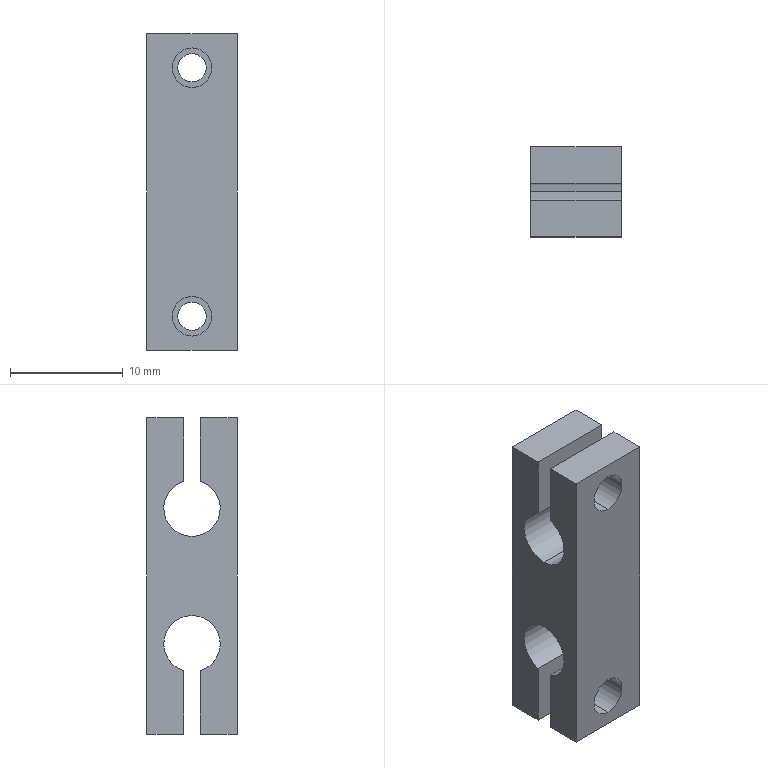Part | STEP file | 06-01-17 laser rotary plate B | 1 solid | 23 faces | box 8 x 8 x 28 mm | volume 1250 mm3 | plane 12 | cylinder 11 | commonest cylinder face diameters 2.5 x4 3.5 x4 5 x3
STEP:
#1=CARTESIAN_POINT('',(0.,0.75,1.75));
#2=VERTEX_POINT('',#1);
#3=CARTESIAN_POINT('',(0.,0.75,4.25));
#4=VERTEX_POINT('',#3);
#5=CARTESIAN_POINT('',(0.,0.75,3.));
#6=DIRECTION('',(0.,1.,0.));
#7=DIRECTION('',(0.,0.,1.));
#8=AXIS2_PLACEMENT_3D('',#5,#6,#7);
#9=CIRCLE('',#8,1.25);
#10=EDGE_CURVE('',#2,#4,#9,.T.);
#11=ORIENTED_EDGE('',*,*,#10,.F.);
#12=CARTESIAN_POINT('',(0.,4.,1.75));
#13=VERTEX_POINT('',#12);
#14=CARTESIAN_POINT('',(0.,4.,1.75));
#15=DIRECTION('',(0.,1.,0.));
#16=VECTOR('',#15,1000.);
#17=LINE('',#14,#16);
#18=EDGE_CURVE('',#2,#13,#17,.T.);
#19=ORIENTED_EDGE('',*,*,#18,.T.);
#20=CARTESIAN_POINT('',(0.,4.,4.25));
#21=VERTEX_POINT('',#20);
#22=CARTESIAN_POINT('',(0.,4.,3.));
#23=DIRECTION('',(0.,1.,0.));
#24=DIRECTION('',(0.,0.,1.));
#25=AXIS2_PLACEMENT_3D('',#22,#23,#24);
#26=CIRCLE('',#25,1.25);
#27=EDGE_CURVE('',#13,#21,#26,.T.);
#28=ORIENTED_EDGE('',*,*,#27,.T.);
#29=CARTESIAN_POINT('',(0.,4.,4.25));
#30=DIRECTION('',(0.,1.,0.));
#31=VECTOR('',#30,1000.);
#32=LINE('',#29,#31);
#33=EDGE_CURVE('',#4,#21,#32,.T.);
#34=ORIENTED_EDGE('',*,*,#33,.F.);
#35=EDGE_LOOP('',(#11,#19,#28,#34));
#36=FACE_OUTER_BOUND('',#35,.T.);
#37=CARTESIAN_POINT('',(0.,4.,3.));
#38=DIRECTION('',(0.,1.,0.));
#39=DIRECTION('',(0.,0.,1.));
#40=AXIS2_PLACEMENT_3D('',#37,#38,#39);
#41=CYLINDRICAL_SURFACE('',#40,1.25);
#42=ADVANCED_FACE('',(#36),#41,.F.);
#43=CARTESIAN_POINT('',(0.,0.75,23.75));
#44=VERTEX_POINT('',#43);
#45=CARTESIAN_POINT('',(0.,0.75,26.25));
#46=VERTEX_POINT('',#45);
#47=CARTESIAN_POINT('',(0.,0.75,25.));
#48=DIRECTION('',(0.,1.,0.));
#49=DIRECTION('',(0.,0.,1.));
#50=AXIS2_PLACEMENT_3D('',#47,#48,#49);
#51=CIRCLE('',#50,1.25);
#52=EDGE_CURVE('',#44,#46,#51,.T.);
#53=ORIENTED_EDGE('',*,*,#52,.F.);
#54=CARTESIAN_POINT('',(0.,4.,23.75));
#55=VERTEX_POINT('',#54);
#56=CARTESIAN_POINT('',(0.,4.,23.75));
#57=DIRECTION('',(0.,1.,0.));
#58=VECTOR('',#57,1000.);
#59=LINE('',#56,#58);
#60=EDGE_CURVE('',#44,#55,#59,.T.);
#61=ORIENTED_EDGE('',*,*,#60,.T.);
#62=CARTESIAN_POINT('',(0.,4.,26.25));
#63=VERTEX_POINT('',#62);
#64=CARTESIAN_POINT('',(0.,4.,25.));
#65=DIRECTION('',(0.,1.,0.));
#66=DIRECTION('',(0.,0.,1.));
#67=AXIS2_PLACEMENT_3D('',#64,#65,#66);
#68=CIRCLE('',#67,1.25);
#69=EDGE_CURVE('',#55,#63,#68,.T.);
#70=ORIENTED_EDGE('',*,*,#69,.T.);
#71=CARTESIAN_POINT('',(0.,4.,26.25));
#72=DIRECTION('',(0.,1.,0.));
#73=VECTOR('',#72,1000.);
#74=LINE('',#71,#73);
#75=EDGE_CURVE('',#46,#63,#74,.T.);
#76=ORIENTED_EDGE('',*,*,#75,.F.);
#77=EDGE_LOOP('',(#53,#61,#70,#76));
#78=FACE_OUTER_BOUND('',#77,.T.);
#79=CARTESIAN_POINT('',(0.,4.,25.));
#80=DIRECTION('',(0.,1.,0.));
#81=DIRECTION('',(0.,0.,1.));
#82=AXIS2_PLACEMENT_3D('',#79,#80,#81);
#83=CYLINDRICAL_SURFACE('',#82,1.25);
#84=ADVANCED_FACE('',(#78),#83,.F.);
#85=CARTESIAN_POINT('',(0.,-0.75,26.75));
#86=VERTEX_POINT('',#85);
#87=CARTESIAN_POINT('',(0.,-0.75,23.25));
#88=VERTEX_POINT('',#87);
#89=CARTESIAN_POINT('',(0.,-0.75,25.));
#90=DIRECTION('',(0.,-1.,0.));
#91=DIRECTION('',(0.,0.,-1.));
#92=AXIS2_PLACEMENT_3D('',#89,#90,#91);
#93=CIRCLE('',#92,1.75);
#94=EDGE_CURVE('',#86,#88,#93,.T.);
#95=ORIENTED_EDGE('',*,*,#94,.F.);
#96=CARTESIAN_POINT('',(0.,-4.,26.75));
#97=VERTEX_POINT('',#96);
#98=CARTESIAN_POINT('',(0.,0.,26.75));
#99=DIRECTION('',(0.,-1.,0.));
#100=VECTOR('',#99,1000.);
#101=LINE('',#98,#100);
#102=EDGE_CURVE('',#86,#97,#101,.T.);
#103=ORIENTED_EDGE('',*,*,#102,.T.);
#104=CARTESIAN_POINT('',(0.,-4.,23.25));
#105=VERTEX_POINT('',#104);
#106=CARTESIAN_POINT('',(0.,-4.,25.));
#107=DIRECTION('',(0.,-1.,0.));
#108=DIRECTION('',(0.,0.,1.));
#109=AXIS2_PLACEMENT_3D('',#106,#107,#108);
#110=CIRCLE('',#109,1.75);
#111=EDGE_CURVE('',#97,#105,#110,.T.);
#112=ORIENTED_EDGE('',*,*,#111,.T.);
#113=CARTESIAN_POINT('',(0.,0.,23.25));
#114=DIRECTION('',(0.,-1.,0.));
#115=VECTOR('',#114,1000.);
#116=LINE('',#113,#115);
#117=EDGE_CURVE('',#88,#105,#116,.T.);
#118=ORIENTED_EDGE('',*,*,#117,.F.);
#119=EDGE_LOOP('',(#95,#103,#112,#118));
#120=FACE_OUTER_BOUND('',#119,.T.);
#121=CARTESIAN_POINT('',(0.,0.,25.));
#122=DIRECTION('',(0.,-1.,0.));
#123=DIRECTION('',(0.,0.,-1.));
#124=AXIS2_PLACEMENT_3D('',#121,#122,#123);
#125=CYLINDRICAL_SURFACE('',#124,1.75);
#126=ADVANCED_FACE('',(#120),#125,.F.);
#127=CARTESIAN_POINT('',(0.,-0.75,4.75));
#128=VERTEX_POINT('',#127);
#129=CARTESIAN_POINT('',(0.,-0.75,1.25));
#130=VERTEX_POINT('',#129);
#131=CARTESIAN_POINT('',(0.,-0.75,3.));
#132=DIRECTION('',(0.,-1.,0.));
#133=DIRECTION('',(0.,0.,-1.));
#134=AXIS2_PLACEMENT_3D('',#131,#132,#133);
#135=CIRCLE('',#134,1.75);
#136=EDGE_CURVE('',#128,#130,#135,.T.);
#137=ORIENTED_EDGE('',*,*,#136,.F.);
#138=CARTESIAN_POINT('',(0.,-4.,4.75));
#139=VERTEX_POINT('',#138);
#140=CARTESIAN_POINT('',(0.,0.,4.75));
#141=DIRECTION('',(0.,-1.,0.));
#142=VECTOR('',#141,1000.);
#143=LINE('',#140,#142);
#144=EDGE_CURVE('',#128,#139,#143,.T.);
#145=ORIENTED_EDGE('',*,*,#144,.T.);
#146=CARTESIAN_POINT('',(0.,-4.,1.25));
#147=VERTEX_POINT('',#146);
#148=CARTESIAN_POINT('',(0.,-4.,3.));
#149=DIRECTION('',(0.,-1.,0.));
#150=DIRECTION('',(0.,0.,-1.));
#151=AXIS2_PLACEMENT_3D('',#148,#149,#150);
#152=CIRCLE('',#151,1.75);
#153=EDGE_CURVE('',#139,#147,#152,.T.);
#154=ORIENTED_EDGE('',*,*,#153,.T.);
#155=CARTESIAN_POINT('',(0.,0.,1.25));
#156=DIRECTION('',(0.,-1.,0.));
#157=VECTOR('',#156,1000.);
#158=LINE('',#155,#157);
#159=EDGE_CURVE('',#130,#147,#158,.T.);
#160=ORIENTED_EDGE('',*,*,#159,.F.);
#161=EDGE_LOOP('',(#137,#145,#154,#160));
#162=FACE_OUTER_BOUND('',#161,.T.);
#163=CARTESIAN_POINT('',(0.,0.,3.));
#164=DIRECTION('',(0.,-1.,0.));
#165=DIRECTION('',(0.,0.,-1.));
#166=AXIS2_PLACEMENT_3D('',#163,#164,#165);
#167=CYLINDRICAL_SURFACE('',#166,1.75);
#168=ADVANCED_FACE('',(#162),#167,.F.);
#169=CARTESIAN_POINT('',(-4.,0.,17.5));
#170=VERTEX_POINT('',#169);
#171=CARTESIAN_POINT('',(-4.,0.75,22.385));
#172=VERTEX_POINT('',#171);
#173=CARTESIAN_POINT('',(-4.,0.,20.));
#174=DIRECTION('',(1.,0.,0.));
#175=DIRECTION('',(0.,0.,-1.));
#176=AXIS2_PLACEMENT_3D('',#173,#174,#175);
#177=CIRCLE('',#176,2.5);
#178=EDGE_CURVE('',#170,#172,#177,.T.);
#179=ORIENTED_EDGE('',*,*,#178,.F.);
#180=CARTESIAN_POINT('',(4.,0.,17.5));
#181=VERTEX_POINT('',#180);
#182=CARTESIAN_POINT('',(-6.,0.,17.5));
#183=DIRECTION('',(1.,0.,0.));
#184=VECTOR('',#183,1000.);
#185=LINE('',#182,#184);
#186=EDGE_CURVE('',#170,#181,#185,.T.);
#187=ORIENTED_EDGE('',*,*,#186,.T.);
#188=CARTESIAN_POINT('',(4.,0.75,22.385));
#189=VERTEX_POINT('',#188);
#190=CARTESIAN_POINT('',(4.,0.,20.));
#191=DIRECTION('',(1.,0.,0.));
#192=DIRECTION('',(0.,0.,-1.));
#193=AXIS2_PLACEMENT_3D('',#190,#191,#192);
#194=CIRCLE('',#193,2.5);
#195=EDGE_CURVE('',#181,#189,#194,.T.);
#196=ORIENTED_EDGE('',*,*,#195,.T.);
#197=CARTESIAN_POINT('',(-6.,0.75,22.385));
#198=DIRECTION('',(-1.,0.,0.));
#199=VECTOR('',#198,1000.);
#200=LINE('',#197,#199);
#201=EDGE_CURVE('',#189,#172,#200,.T.);
#202=ORIENTED_EDGE('',*,*,#201,.T.);
#203=EDGE_LOOP('',(#179,#187,#196,#202));
#204=FACE_OUTER_BOUND('',#203,.T.);
#205=CARTESIAN_POINT('',(-6.,0.,20.));
#206=DIRECTION('',(1.,0.,0.));
#207=DIRECTION('',(0.,0.,-1.));
#208=AXIS2_PLACEMENT_3D('',#205,#206,#207);
#209=CYLINDRICAL_SURFACE('',#208,2.5);
#210=ADVANCED_FACE('',(#204),#209,.F.);
#211=CARTESIAN_POINT('',(4.,0.75,28.));
#212=VERTEX_POINT('',#211);
#213=CARTESIAN_POINT('',(-4.,0.75,28.));
#214=VERTEX_POINT('',#213);
#215=CARTESIAN_POINT('',(4.,0.75,28.));
#216=DIRECTION('',(-1.,0.,0.));
#217=VECTOR('',#216,1000.);
#218=LINE('',#215,#217);
#219=EDGE_CURVE('',#212,#214,#218,.T.);
#220=ORIENTED_EDGE('',*,*,#219,.F.);
#221=CARTESIAN_POINT('',(4.,4.,28.));
#222=VERTEX_POINT('',#221);
#223=CARTESIAN_POINT('',(4.,4.,28.));
#224=DIRECTION('',(0.,1.,0.));
#225=VECTOR('',#224,1000.);
#226=LINE('',#223,#225);
#227=EDGE_CURVE('',#212,#222,#226,.T.);
#228=ORIENTED_EDGE('',*,*,#227,.T.);
#229=CARTESIAN_POINT('',(-4.,4.,28.));
#230=VERTEX_POINT('',#229);
#231=CARTESIAN_POINT('',(-4.,4.,28.));
#232=DIRECTION('',(-1.,0.,0.));
#233=VECTOR('',#232,1000.);
#234=LINE('',#231,#233);
#235=EDGE_CURVE('',#222,#230,#234,.T.);
#236=ORIENTED_EDGE('',*,*,#235,.T.);
#237=CARTESIAN_POINT('',(-4.,4.,28.));
#238=DIRECTION('',(0.,-1.,0.));
#239=VECTOR('',#238,1000.);
#240=LINE('',#237,#239);
#241=EDGE_CURVE('',#230,#214,#240,.T.);
#242=ORIENTED_EDGE('',*,*,#241,.T.);
#243=EDGE_LOOP('',(#220,#228,#236,#242));
#244=FACE_OUTER_BOUND('',#243,.T.);
#245=CARTESIAN_POINT('',(4.,-4.,28.));
#246=DIRECTION('',(0.,0.,1.));
#247=DIRECTION('',(1.,0.,0.));
#248=AXIS2_PLACEMENT_3D('',#245,#246,#247);
#249=PLANE('',#248);
#250=ADVANCED_FACE('',(#244),#249,.T.);
#251=CARTESIAN_POINT('',(4.,0.75,0.));
#252=VERTEX_POINT('',#251);
#253=CARTESIAN_POINT('',(4.,4.,0.));
#254=VERTEX_POINT('',#253);
#255=CARTESIAN_POINT('',(4.,4.,0.));
#256=DIRECTION('',(0.,1.,0.));
#257=VECTOR('',#256,1000.);
#258=LINE('',#255,#257);
#259=EDGE_CURVE('',#252,#254,#258,.T.);
#260=ORIENTED_EDGE('',*,*,#259,.F.);
#261=CARTESIAN_POINT('',(-4.,0.75,0.));
#262=VERTEX_POINT('',#261);
#263=CARTESIAN_POINT('',(4.,0.75,0.));
#264=DIRECTION('',(-1.,0.,0.));
#265=VECTOR('',#264,1000.);
#266=LINE('',#263,#265);
#267=EDGE_CURVE('',#252,#262,#266,.T.);
#268=ORIENTED_EDGE('',*,*,#267,.T.);
#269=CARTESIAN_POINT('',(-4.,4.,0.));
#270=VERTEX_POINT('',#269);
#271=CARTESIAN_POINT('',(-4.,4.,0.));
#272=DIRECTION('',(0.,-1.,0.));
#273=VECTOR('',#272,1000.);
#274=LINE('',#271,#273);
#275=EDGE_CURVE('',#270,#262,#274,.T.);
#276=ORIENTED_EDGE('',*,*,#275,.F.);
#277=CARTESIAN_POINT('',(-4.,4.,0.));
#278=DIRECTION('',(-1.,0.,0.));
#279=VECTOR('',#278,1000.);
#280=LINE('',#277,#279);
#281=EDGE_CURVE('',#254,#270,#280,.T.);
#282=ORIENTED_EDGE('',*,*,#281,.F.);
#283=EDGE_LOOP('',(#260,#268,#276,#282));
#284=FACE_OUTER_BOUND('',#283,.T.);
#285=CARTESIAN_POINT('',(4.,-4.,0.));
#286=DIRECTION('',(0.,0.,1.));
#287=DIRECTION('',(1.,0.,0.));
#288=AXIS2_PLACEMENT_3D('',#285,#286,#287);
#289=PLANE('',#288);
#290=ADVANCED_FACE('',(#284),#289,.F.);
#291=ORIENTED_EDGE('',*,*,#227,.F.);
#292=CARTESIAN_POINT('',(4.,0.75,21.134));
#293=DIRECTION('',(0.,0.,1.));
#294=VECTOR('',#293,1000.);
#295=LINE('',#292,#294);
#296=EDGE_CURVE('',#189,#212,#295,.T.);
#297=ORIENTED_EDGE('',*,*,#296,.F.);
#298=ORIENTED_EDGE('',*,*,#195,.F.);
#299=CARTESIAN_POINT('',(4.,-0.75,22.385));
#300=VERTEX_POINT('',#299);
#301=CARTESIAN_POINT('',(4.,0.,20.));
#302=DIRECTION('',(1.,0.,0.));
#303=DIRECTION('',(0.,0.,-1.));
#304=AXIS2_PLACEMENT_3D('',#301,#302,#303);
#305=CIRCLE('',#304,2.5);
#306=EDGE_CURVE('',#300,#181,#305,.T.);
#307=ORIENTED_EDGE('',*,*,#306,.F.);
#308=CARTESIAN_POINT('',(4.,-0.75,28.));
#309=VERTEX_POINT('',#308);
#310=CARTESIAN_POINT('',(4.,-0.75,21.134));
#311=DIRECTION('',(0.,0.,-1.));
#312=VECTOR('',#311,1000.);
#313=LINE('',#310,#312);
#314=EDGE_CURVE('',#309,#300,#313,.T.);
#315=ORIENTED_EDGE('',*,*,#314,.F.);
#316=CARTESIAN_POINT('',(4.,-4.,28.));
#317=VERTEX_POINT('',#316);
#318=CARTESIAN_POINT('',(4.,4.,28.));
#319=DIRECTION('',(0.,1.,0.));
#320=VECTOR('',#319,1000.);
#321=LINE('',#318,#320);
#322=EDGE_CURVE('',#317,#309,#321,.T.);
#323=ORIENTED_EDGE('',*,*,#322,.F.);
#324=CARTESIAN_POINT('',(4.,-4.,0.));
#325=VERTEX_POINT('',#324);
#326=CARTESIAN_POINT('',(4.,-4.,28.));
#327=DIRECTION('',(0.,0.,-1.));
#328=VECTOR('',#327,1000.);
#329=LINE('',#326,#328);
#330=EDGE_CURVE('',#317,#325,#329,.T.);
#331=ORIENTED_EDGE('',*,*,#330,.T.);
#332=CARTESIAN_POINT('',(4.,-0.75,0.));
#333=VERTEX_POINT('',#332);
#334=CARTESIAN_POINT('',(4.,4.,0.));
#335=DIRECTION('',(0.,1.,0.));
#336=VECTOR('',#335,1000.);
#337=LINE('',#334,#336);
#338=EDGE_CURVE('',#325,#333,#337,.T.);
#339=ORIENTED_EDGE('',*,*,#338,.T.);
#340=CARTESIAN_POINT('',(4.,-0.75,5.615));
#341=VERTEX_POINT('',#340);
#342=CARTESIAN_POINT('',(4.,-0.75,6.866));
#343=DIRECTION('',(0.,0.,-1.));
#344=VECTOR('',#343,1000.);
#345=LINE('',#342,#344);
#346=EDGE_CURVE('',#341,#333,#345,.T.);
#347=ORIENTED_EDGE('',*,*,#346,.F.);
#348=CARTESIAN_POINT('',(4.,0.75,5.615));
#349=VERTEX_POINT('',#348);
#350=CARTESIAN_POINT('',(4.,0.,8.));
#351=DIRECTION('',(1.,0.,0.));
#352=DIRECTION('',(0.,0.,-1.));
#353=AXIS2_PLACEMENT_3D('',#350,#351,#352);
#354=CIRCLE('',#353,2.5);
#355=EDGE_CURVE('',#349,#341,#354,.T.);
#356=ORIENTED_EDGE('',*,*,#355,.F.);
#357=CARTESIAN_POINT('',(4.,0.75,6.866));
#358=DIRECTION('',(0.,0.,1.));
#359=VECTOR('',#358,1000.);
#360=LINE('',#357,#359);
#361=EDGE_CURVE('',#252,#349,#360,.T.);
#362=ORIENTED_EDGE('',*,*,#361,.F.);
#363=ORIENTED_EDGE('',*,*,#259,.T.);
#364=CARTESIAN_POINT('',(4.,4.,28.));
#365=DIRECTION('',(0.,0.,-1.));
#366=VECTOR('',#365,1000.);
#367=LINE('',#364,#366);
#368=EDGE_CURVE('',#222,#254,#367,.T.);
#369=ORIENTED_EDGE('',*,*,#368,.F.);
#370=EDGE_LOOP('',(#291,#297,#298,#307,#315,#323,#331,#339,#347,#356,#362,#363,#369));
#371=FACE_OUTER_BOUND('',#370,.T.);
#372=CARTESIAN_POINT('',(4.,4.,28.));
#373=DIRECTION('',(-1.,0.,0.));
#374=DIRECTION('',(0.,0.,1.));
#375=AXIS2_PLACEMENT_3D('',#372,#373,#374);
#376=PLANE('',#375);
#377=ADVANCED_FACE('',(#371),#376,.F.);
#378=CARTESIAN_POINT('',(0.,4.,3.));
#379=DIRECTION('',(0.,1.,0.));
#380=DIRECTION('',(0.,0.,1.));
#381=AXIS2_PLACEMENT_3D('',#378,#379,#380);
#382=CIRCLE('',#381,1.25);
#383=EDGE_CURVE('',#21,#13,#382,.T.);
#384=ORIENTED_EDGE('',*,*,#383,.F.);
#385=ORIENTED_EDGE('',*,*,#27,.F.);
#386=EDGE_LOOP('',(#384,#385));
#387=FACE_BOUND('',#386,.T.);
#388=CARTESIAN_POINT('',(0.,4.,25.));
#389=DIRECTION('',(0.,1.,0.));
#390=DIRECTION('',(0.,0.,1.));
#391=AXIS2_PLACEMENT_3D('',#388,#389,#390);
#392=CIRCLE('',#391,1.25);
#393=EDGE_CURVE('',#63,#55,#392,.T.);
#394=ORIENTED_EDGE('',*,*,#393,.F.);
#395=ORIENTED_EDGE('',*,*,#69,.F.);
#396=EDGE_LOOP('',(#394,#395));
#397=FACE_BOUND('',#396,.T.);
#398=ORIENTED_EDGE('',*,*,#281,.T.);
#399=CARTESIAN_POINT('',(-4.,4.,28.));
#400=DIRECTION('',(0.,0.,-1.));
#401=VECTOR('',#400,1000.);
#402=LINE('',#399,#401);
#403=EDGE_CURVE('',#230,#270,#402,.T.);
#404=ORIENTED_EDGE('',*,*,#403,.F.);
#405=ORIENTED_EDGE('',*,*,#235,.F.);
#406=ORIENTED_EDGE('',*,*,#368,.T.);
#407=EDGE_LOOP('',(#398,#404,#405,#406));
#408=FACE_OUTER_BOUND('',#407,.T.);
#409=CARTESIAN_POINT('',(-4.,4.,28.));
#410=DIRECTION('',(0.,-1.,0.));
#411=DIRECTION('',(0.,0.,-1.));
#412=AXIS2_PLACEMENT_3D('',#409,#410,#411);
#413=PLANE('',#412);
#414=ADVANCED_FACE('',(#387,#397,#408),#413,.F.);
#415=CARTESIAN_POINT('',(-4.,-0.75,22.385));
#416=VERTEX_POINT('',#415);
#417=CARTESIAN_POINT('',(-4.,0.,20.));
#418=DIRECTION('',(1.,0.,0.));
#419=DIRECTION('',(0.,0.,-1.));
#420=AXIS2_PLACEMENT_3D('',#417,#418,#419);
#421=CIRCLE('',#420,2.5);
#422=EDGE_CURVE('',#416,#170,#421,.T.);
#423=ORIENTED_EDGE('',*,*,#422,.T.);
#424=ORIENTED_EDGE('',*,*,#178,.T.);
#425=CARTESIAN_POINT('',(-4.,0.75,28.));
#426=DIRECTION('',(0.,0.,1.));
#427=VECTOR('',#426,1000.);
#428=LINE('',#425,#427);
#429=EDGE_CURVE('',#172,#214,#428,.T.);
#430=ORIENTED_EDGE('',*,*,#429,.T.);
#431=ORIENTED_EDGE('',*,*,#241,.F.);
#432=ORIENTED_EDGE('',*,*,#403,.T.);
#433=ORIENTED_EDGE('',*,*,#275,.T.);
#434=CARTESIAN_POINT('',(-4.,0.75,5.615));
#435=VERTEX_POINT('',#434);
#436=CARTESIAN_POINT('',(-4.,0.75,28.));
#437=DIRECTION('',(0.,0.,1.));
#438=VECTOR('',#437,1000.);
#439=LINE('',#436,#438);
#440=EDGE_CURVE('',#262,#435,#439,.T.);
#441=ORIENTED_EDGE('',*,*,#440,.T.);
#442=CARTESIAN_POINT('',(-4.,-0.75,5.615));
#443=VERTEX_POINT('',#442);
#444=CARTESIAN_POINT('',(-4.,0.,8.));
#445=DIRECTION('',(1.,0.,0.));
#446=DIRECTION('',(0.,0.,-1.));
#447=AXIS2_PLACEMENT_3D('',#444,#445,#446);
#448=CIRCLE('',#447,2.5);
#449=EDGE_CURVE('',#435,#443,#448,.T.);
#450=ORIENTED_EDGE('',*,*,#449,.T.);
#451=CARTESIAN_POINT('',(-4.,-0.75,0.));
#452=VERTEX_POINT('',#451);
#453=CARTESIAN_POINT('',(-4.,-0.75,28.));
#454=DIRECTION('',(0.,0.,-1.));
#455=VECTOR('',#454,1000.);
#456=LINE('',#453,#455);
#457=EDGE_CURVE('',#443,#452,#456,.T.);
#458=ORIENTED_EDGE('',*,*,#457,.T.);
#459=CARTESIAN_POINT('',(-4.,-4.,0.));
#460=VERTEX_POINT('',#459);
#461=CARTESIAN_POINT('',(-4.,4.,0.));
#462=DIRECTION('',(0.,-1.,0.));
#463=VECTOR('',#462,1000.);
#464=LINE('',#461,#463);
#465=EDGE_CURVE('',#452,#460,#464,.T.);
#466=ORIENTED_EDGE('',*,*,#465,.T.);
#467=CARTESIAN_POINT('',(-4.,-4.,28.));
#468=VERTEX_POINT('',#467);
#469=CARTESIAN_POINT('',(-4.,-4.,28.));
#470=DIRECTION('',(0.,0.,-1.));
#471=VECTOR('',#470,1000.);
#472=LINE('',#469,#471);
#473=EDGE_CURVE('',#468,#460,#472,.T.);
#474=ORIENTED_EDGE('',*,*,#473,.F.);
#475=CARTESIAN_POINT('',(-4.,-0.75,28.));
#476=VERTEX_POINT('',#475);
#477=CARTESIAN_POINT('',(-4.,4.,28.));
#478=DIRECTION('',(0.,-1.,0.));
#479=VECTOR('',#478,1000.);
#480=LINE('',#477,#479);
#481=EDGE_CURVE('',#476,#468,#480,.T.);
#482=ORIENTED_EDGE('',*,*,#481,.F.);
#483=CARTESIAN_POINT('',(-4.,-0.75,28.));
#484=DIRECTION('',(0.,0.,-1.));
#485=VECTOR('',#484,1000.);
#486=LINE('',#483,#485);
#487=EDGE_CURVE('',#476,#416,#486,.T.);
#488=ORIENTED_EDGE('',*,*,#487,.T.);
#489=EDGE_LOOP('',(#423,#424,#430,#431,#432,#433,#441,#450,#458,#466,#474,#482,#488));
#490=FACE_OUTER_BOUND('',#489,.T.);
#491=CARTESIAN_POINT('',(-4.,4.,28.));
#492=DIRECTION('',(1.,0.,0.));
#493=DIRECTION('',(0.,0.,-1.));
#494=AXIS2_PLACEMENT_3D('',#491,#492,#493);
#495=PLANE('',#494);
#496=ADVANCED_FACE('',(#490),#495,.F.);
#497=CARTESIAN_POINT('',(0.,-4.,25.));
#498=DIRECTION('',(0.,-1.,0.));
#499=DIRECTION('',(0.,0.,1.));
#500=AXIS2_PLACEMENT_3D('',#497,#498,#499);
#501=CIRCLE('',#500,1.75);
#502=EDGE_CURVE('',#105,#97,#501,.T.);
#503=ORIENTED_EDGE('',*,*,#502,.F.);
#504=ORIENTED_EDGE('',*,*,#111,.F.);
#505=EDGE_LOOP('',(#503,#504));
#506=FACE_BOUND('',#505,.T.);
#507=CARTESIAN_POINT('',(0.,-4.,3.));
#508=DIRECTION('',(0.,-1.,0.));
#509=DIRECTION('',(0.,0.,-1.));
#510=AXIS2_PLACEMENT_3D('',#507,#508,#509);
#511=CIRCLE('',#510,1.75);
#512=EDGE_CURVE('',#147,#139,#511,.T.);
#513=ORIENTED_EDGE('',*,*,#512,.F.);
#514=ORIENTED_EDGE('',*,*,#153,.F.);
#515=EDGE_LOOP('',(#513,#514));
#516=FACE_BOUND('',#515,.T.);
#517=CARTESIAN_POINT('',(-4.,-4.,0.));
#518=DIRECTION('',(1.,0.,0.));
#519=VECTOR('',#518,1000.);
#520=LINE('',#517,#519);
#521=EDGE_CURVE('',#460,#325,#520,.T.);
#522=ORIENTED_EDGE('',*,*,#521,.T.);
#523=ORIENTED_EDGE('',*,*,#330,.F.);
#524=CARTESIAN_POINT('',(-4.,-4.,28.));
#525=DIRECTION('',(1.,0.,0.));
#526=VECTOR('',#525,1000.);
#527=LINE('',#524,#526);
#528=EDGE_CURVE('',#468,#317,#527,.T.);
#529=ORIENTED_EDGE('',*,*,#528,.F.);
#530=ORIENTED_EDGE('',*,*,#473,.T.);
#531=EDGE_LOOP('',(#522,#523,#529,#530));
#532=FACE_OUTER_BOUND('',#531,.T.);
#533=CARTESIAN_POINT('',(-4.,-4.,28.));
#534=DIRECTION('',(0.,1.,0.));
#535=DIRECTION('',(0.,0.,1.));
#536=AXIS2_PLACEMENT_3D('',#533,#534,#535);
#537=PLANE('',#536);
#538=ADVANCED_FACE('',(#506,#516,#532),#537,.F.);
#539=CARTESIAN_POINT('',(4.,-0.75,28.));
#540=DIRECTION('',(1.,0.,0.));
#541=VECTOR('',#540,1000.);
#542=LINE('',#539,#541);
#543=EDGE_CURVE('',#476,#309,#542,.T.);
#544=ORIENTED_EDGE('',*,*,#543,.F.);
#545=ORIENTED_EDGE('',*,*,#481,.T.);
#546=ORIENTED_EDGE('',*,*,#528,.T.);
#547=ORIENTED_EDGE('',*,*,#322,.T.);
#548=EDGE_LOOP('',(#544,#545,#546,#547));
#549=FACE_OUTER_BOUND('',#548,.T.);
#550=CARTESIAN_POINT('',(4.,-4.,28.));
#551=DIRECTION('',(0.,0.,1.));
#552=DIRECTION('',(1.,0.,0.));
#553=AXIS2_PLACEMENT_3D('',#550,#551,#552);
#554=PLANE('',#553);
#555=ADVANCED_FACE('',(#549),#554,.T.);
#556=ORIENTED_EDGE('',*,*,#465,.F.);
#557=CARTESIAN_POINT('',(4.,-0.75,0.));
#558=DIRECTION('',(1.,0.,0.));
#559=VECTOR('',#558,1000.);
#560=LINE('',#557,#559);
#561=EDGE_CURVE('',#452,#333,#560,.T.);
#562=ORIENTED_EDGE('',*,*,#561,.T.);
#563=ORIENTED_EDGE('',*,*,#338,.F.);
#564=ORIENTED_EDGE('',*,*,#521,.F.);
#565=EDGE_LOOP('',(#556,#562,#563,#564));
#566=FACE_OUTER_BOUND('',#565,.T.);
#567=CARTESIAN_POINT('',(4.,-4.,0.));
#568=DIRECTION('',(0.,0.,1.));
#569=DIRECTION('',(1.,0.,0.));
#570=AXIS2_PLACEMENT_3D('',#567,#568,#569);
#571=PLANE('',#570);
#572=ADVANCED_FACE('',(#566),#571,.F.);
#573=ORIENTED_EDGE('',*,*,#449,.F.);
#574=CARTESIAN_POINT('',(-6.,0.75,5.615));
#575=DIRECTION('',(1.,0.,0.));
#576=VECTOR('',#575,1000.);
#577=LINE('',#574,#576);
#578=EDGE_CURVE('',#435,#349,#577,.T.);
#579=ORIENTED_EDGE('',*,*,#578,.T.);
#580=ORIENTED_EDGE('',*,*,#355,.T.);
#581=CARTESIAN_POINT('',(-6.,-0.75,5.615));
#582=DIRECTION('',(-1.,0.,0.));
#583=VECTOR('',#582,1000.);
#584=LINE('',#581,#583);
#585=EDGE_CURVE('',#341,#443,#584,.T.);
#586=ORIENTED_EDGE('',*,*,#585,.T.);
#587=EDGE_LOOP('',(#573,#579,#580,#586));
#588=FACE_OUTER_BOUND('',#587,.T.);
#589=CARTESIAN_POINT('',(-6.,0.,8.));
#590=DIRECTION('',(1.,0.,0.));
#591=DIRECTION('',(0.,0.,-1.));
#592=AXIS2_PLACEMENT_3D('',#589,#590,#591);
#593=CYLINDRICAL_SURFACE('',#592,2.5);
#594=ADVANCED_FACE('',(#588),#593,.F.);
#595=ORIENTED_EDGE('',*,*,#186,.F.);
#596=ORIENTED_EDGE('',*,*,#422,.F.);
#597=CARTESIAN_POINT('',(-6.,-0.75,22.385));
#598=DIRECTION('',(1.,0.,0.));
#599=VECTOR('',#598,1000.);
#600=LINE('',#597,#599);
#601=EDGE_CURVE('',#416,#300,#600,.T.);
#602=ORIENTED_EDGE('',*,*,#601,.T.);
#603=ORIENTED_EDGE('',*,*,#306,.T.);
#604=EDGE_LOOP('',(#595,#596,#602,#603));
#605=FACE_OUTER_BOUND('',#604,.T.);
#606=CARTESIAN_POINT('',(-6.,0.,20.));
#607=DIRECTION('',(1.,0.,0.));
#608=DIRECTION('',(0.,0.,-1.));
#609=AXIS2_PLACEMENT_3D('',#606,#607,#608);
#610=CYLINDRICAL_SURFACE('',#609,2.5);
#611=ADVANCED_FACE('',(#605),#610,.F.);
#612=CARTESIAN_POINT('',(0.,-0.75,3.));
#613=DIRECTION('',(0.,-1.,0.));
#614=DIRECTION('',(0.,0.,-1.));
#615=AXIS2_PLACEMENT_3D('',#612,#613,#614);
#616=CIRCLE('',#615,1.75);
#617=EDGE_CURVE('',#130,#128,#616,.T.);
#618=ORIENTED_EDGE('',*,*,#617,.T.);
#619=ORIENTED_EDGE('',*,*,#136,.T.);
#620=EDGE_LOOP('',(#618,#619));
#621=FACE_BOUND('',#620,.T.);
#622=ORIENTED_EDGE('',*,*,#457,.F.);
#623=ORIENTED_EDGE('',*,*,#585,.F.);
#624=ORIENTED_EDGE('',*,*,#346,.T.);
#625=ORIENTED_EDGE('',*,*,#561,.F.);
#626=EDGE_LOOP('',(#622,#623,#624,#625));
#627=FACE_OUTER_BOUND('',#626,.T.);
#628=CARTESIAN_POINT('',(-6.,-0.75,6.866));
#629=DIRECTION('',(0.,-1.,0.));
#630=DIRECTION('',(0.,0.,-1.));
#631=AXIS2_PLACEMENT_3D('',#628,#629,#630);
#632=PLANE('',#631);
#633=ADVANCED_FACE('',(#621,#627),#632,.F.);
#634=CARTESIAN_POINT('',(0.,0.75,3.));
#635=DIRECTION('',(0.,1.,0.));
#636=DIRECTION('',(0.,0.,1.));
#637=AXIS2_PLACEMENT_3D('',#634,#635,#636);
#638=CIRCLE('',#637,1.25);
#639=EDGE_CURVE('',#4,#2,#638,.T.);
#640=ORIENTED_EDGE('',*,*,#639,.T.);
#641=ORIENTED_EDGE('',*,*,#10,.T.);
#642=EDGE_LOOP('',(#640,#641));
#643=FACE_BOUND('',#642,.T.);
#644=ORIENTED_EDGE('',*,*,#361,.T.);
#645=ORIENTED_EDGE('',*,*,#578,.F.);
#646=ORIENTED_EDGE('',*,*,#440,.F.);
#647=ORIENTED_EDGE('',*,*,#267,.F.);
#648=EDGE_LOOP('',(#644,#645,#646,#647));
#649=FACE_OUTER_BOUND('',#648,.T.);
#650=CARTESIAN_POINT('',(-6.,0.75,6.866));
#651=DIRECTION('',(0.,1.,0.));
#652=DIRECTION('',(0.,0.,1.));
#653=AXIS2_PLACEMENT_3D('',#650,#651,#652);
#654=PLANE('',#653);
#655=ADVANCED_FACE('',(#643,#649),#654,.F.);
#656=CARTESIAN_POINT('',(0.,-0.75,25.));
#657=DIRECTION('',(0.,-1.,0.));
#658=DIRECTION('',(0.,0.,-1.));
#659=AXIS2_PLACEMENT_3D('',#656,#657,#658);
#660=CIRCLE('',#659,1.75);
#661=EDGE_CURVE('',#88,#86,#660,.T.);
#662=ORIENTED_EDGE('',*,*,#661,.T.);
#663=ORIENTED_EDGE('',*,*,#94,.T.);
#664=EDGE_LOOP('',(#662,#663));
#665=FACE_BOUND('',#664,.T.);
#666=ORIENTED_EDGE('',*,*,#543,.T.);
#667=ORIENTED_EDGE('',*,*,#314,.T.);
#668=ORIENTED_EDGE('',*,*,#601,.F.);
#669=ORIENTED_EDGE('',*,*,#487,.F.);
#670=EDGE_LOOP('',(#666,#667,#668,#669));
#671=FACE_OUTER_BOUND('',#670,.T.);
#672=CARTESIAN_POINT('',(-6.,-0.75,21.134));
#673=DIRECTION('',(0.,-1.,0.));
#674=DIRECTION('',(0.,0.,-1.));
#675=AXIS2_PLACEMENT_3D('',#672,#673,#674);
#676=PLANE('',#675);
#677=ADVANCED_FACE('',(#665,#671),#676,.F.);
#678=CARTESIAN_POINT('',(0.,0.75,25.));
#679=DIRECTION('',(0.,1.,0.));
#680=DIRECTION('',(0.,0.,1.));
#681=AXIS2_PLACEMENT_3D('',#678,#679,#680);
#682=CIRCLE('',#681,1.25);
#683=EDGE_CURVE('',#46,#44,#682,.T.);
#684=ORIENTED_EDGE('',*,*,#683,.T.);
#685=ORIENTED_EDGE('',*,*,#52,.T.);
#686=EDGE_LOOP('',(#684,#685));
#687=FACE_BOUND('',#686,.T.);
#688=ORIENTED_EDGE('',*,*,#219,.T.);
#689=ORIENTED_EDGE('',*,*,#429,.F.);
#690=ORIENTED_EDGE('',*,*,#201,.F.);
#691=ORIENTED_EDGE('',*,*,#296,.T.);
#692=EDGE_LOOP('',(#688,#689,#690,#691));
#693=FACE_OUTER_BOUND('',#692,.T.);
#694=CARTESIAN_POINT('',(-6.,0.75,21.134));
#695=DIRECTION('',(0.,1.,0.));
#696=DIRECTION('',(0.,0.,1.));
#697=AXIS2_PLACEMENT_3D('',#694,#695,#696);
#698=PLANE('',#697);
#699=ADVANCED_FACE('',(#687,#693),#698,.F.);
#700=ORIENTED_EDGE('',*,*,#144,.F.);
#701=ORIENTED_EDGE('',*,*,#617,.F.);
#702=ORIENTED_EDGE('',*,*,#159,.T.);
#703=ORIENTED_EDGE('',*,*,#512,.T.);
#704=EDGE_LOOP('',(#700,#701,#702,#703));
#705=FACE_OUTER_BOUND('',#704,.T.);
#706=CARTESIAN_POINT('',(0.,0.,3.));
#707=DIRECTION('',(0.,-1.,0.));
#708=DIRECTION('',(0.,0.,-1.));
#709=AXIS2_PLACEMENT_3D('',#706,#707,#708);
#710=CYLINDRICAL_SURFACE('',#709,1.75);
#711=ADVANCED_FACE('',(#705),#710,.F.);
#712=ORIENTED_EDGE('',*,*,#102,.F.);
#713=ORIENTED_EDGE('',*,*,#661,.F.);
#714=ORIENTED_EDGE('',*,*,#117,.T.);
#715=ORIENTED_EDGE('',*,*,#502,.T.);
#716=EDGE_LOOP('',(#712,#713,#714,#715));
#717=FACE_OUTER_BOUND('',#716,.T.);
#718=CARTESIAN_POINT('',(0.,0.,25.));
#719=DIRECTION('',(0.,-1.,0.));
#720=DIRECTION('',(0.,0.,-1.));
#721=AXIS2_PLACEMENT_3D('',#718,#719,#720);
#722=CYLINDRICAL_SURFACE('',#721,1.75);
#723=ADVANCED_FACE('',(#717),#722,.F.);
#724=ORIENTED_EDGE('',*,*,#60,.F.);
#725=ORIENTED_EDGE('',*,*,#683,.F.);
#726=ORIENTED_EDGE('',*,*,#75,.T.);
#727=ORIENTED_EDGE('',*,*,#393,.T.);
#728=EDGE_LOOP('',(#724,#725,#726,#727));
#729=FACE_OUTER_BOUND('',#728,.T.);
#730=CARTESIAN_POINT('',(0.,4.,25.));
#731=DIRECTION('',(0.,1.,0.));
#732=DIRECTION('',(0.,0.,1.));
#733=AXIS2_PLACEMENT_3D('',#730,#731,#732);
#734=CYLINDRICAL_SURFACE('',#733,1.25);
#735=ADVANCED_FACE('',(#729),#734,.F.);
#736=ORIENTED_EDGE('',*,*,#18,.F.);
#737=ORIENTED_EDGE('',*,*,#639,.F.);
#738=ORIENTED_EDGE('',*,*,#33,.T.);
#739=ORIENTED_EDGE('',*,*,#383,.T.);
#740=EDGE_LOOP('',(#736,#737,#738,#739));
#741=FACE_OUTER_BOUND('',#740,.T.);
#742=CARTESIAN_POINT('',(0.,4.,3.));
#743=DIRECTION('',(0.,1.,0.));
#744=DIRECTION('',(0.,0.,1.));
#745=AXIS2_PLACEMENT_3D('',#742,#743,#744);
#746=CYLINDRICAL_SURFACE('',#745,1.25);
#747=ADVANCED_FACE('',(#741),#746,.F.);
#748=CLOSED_SHELL('',(#42,#84,#126,#168,#210,#250,#290,#377,#414,#496,#538,#555,#572,#594,#611,#633,#655,#677,#699,#711,#723,#735,#747));
#749=MANIFOLD_SOLID_BREP('',#748);
#750=CARTESIAN_POINT('',(0.,0.,0.));
#751=DIRECTION('',(0.,0.,1.));
#752=DIRECTION('',(1.,0.,0.));
#753=AXIS2_PLACEMENT_3D('',#750,#751,#752);
#754=(LENGTH_UNIT()NAMED_UNIT(*)SI_UNIT(.MILLI.,.METRE.));
#755=UNCERTAINTY_MEASURE_WITH_UNIT(LENGTH_MEASURE(0.00001),#754,'','');
#756=(NAMED_UNIT(*)PLANE_ANGLE_UNIT()SI_UNIT($,.RADIAN.));
#757=(NAMED_UNIT(*)SI_UNIT($,.STERADIAN.)SOLID_ANGLE_UNIT());
#758=(GEOMETRIC_REPRESENTATION_CONTEXT(3)GLOBAL_UNCERTAINTY_ASSIGNED_CONTEXT((#755))GLOBAL_UNIT_ASSIGNED_CONTEXT((#754,#756,#757))REPRESENTATION_CONTEXT('',''));
#759=ADVANCED_BREP_SHAPE_REPRESENTATION('',(#749,#753),#758);